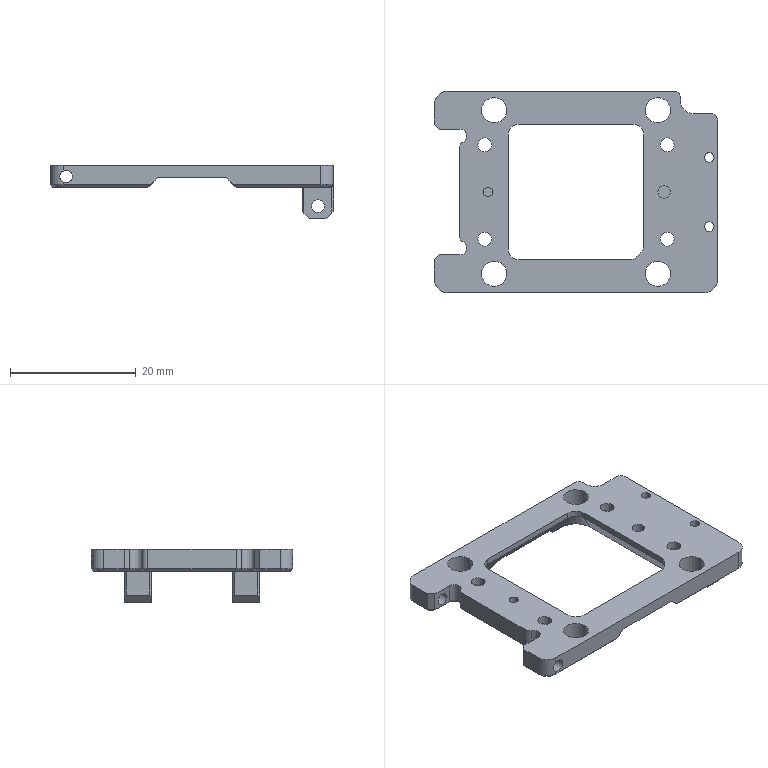NC program | NX | posted with a generic post | part box 45 x 32 x 8.5 mm
Whole program:
N10 G17 G21 G94 G90
(DRILLING_COPY , TOOL : D4A45)
N12 T14 M6
N14 G54
N16 G17 G0 G90 X-20. Y-6.5 B0. C0. S5000 M3
N18 G43 Z30. H14
N20 G94 G81 G98 Z-6.35 F250. R-2.25
N22 X20. Y-1.8 Z-1.1 R3.
N24 G80
N26 G0 X20. Y-1.8 Z30.
N28 M5
(DRILLING_COPY_COPY_COPY_1 , TOOL : 2.02ZT)
N30 T18 M6
N32 G54
N34 G17 G0 G90 X-20. Y-6.5 B0. C0. S1447 M3
N36 G43 Z30. H18
N38 G94 G83 G98 Z-11.607 F100. Q2. R-2.25
N40 X20. Y-1.8 Z-8.107 R3.
N42 G80
N44 G0 X20. Y-1.8 Z30.
N46 M5
N48 M2